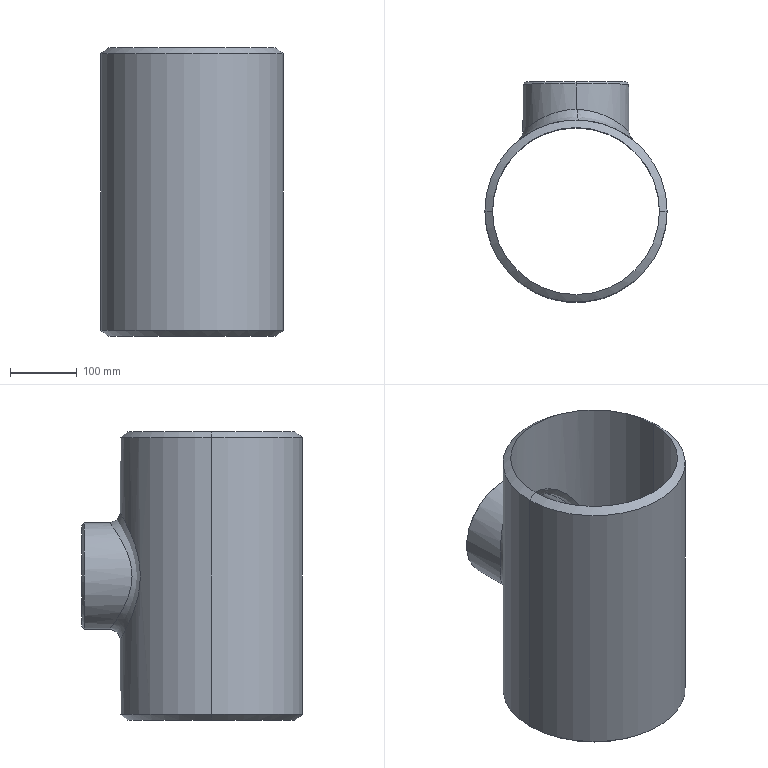Part | NX | features BREP 1 | 1 solid | 18 faces | box 273 x 330.5 x 432 mm | volume 3935888 mm3 | cylinder 8 | cone 6 | spline 4 | commonest cylinder face diameters 150 x2 159 x2 250 x2 273 x2